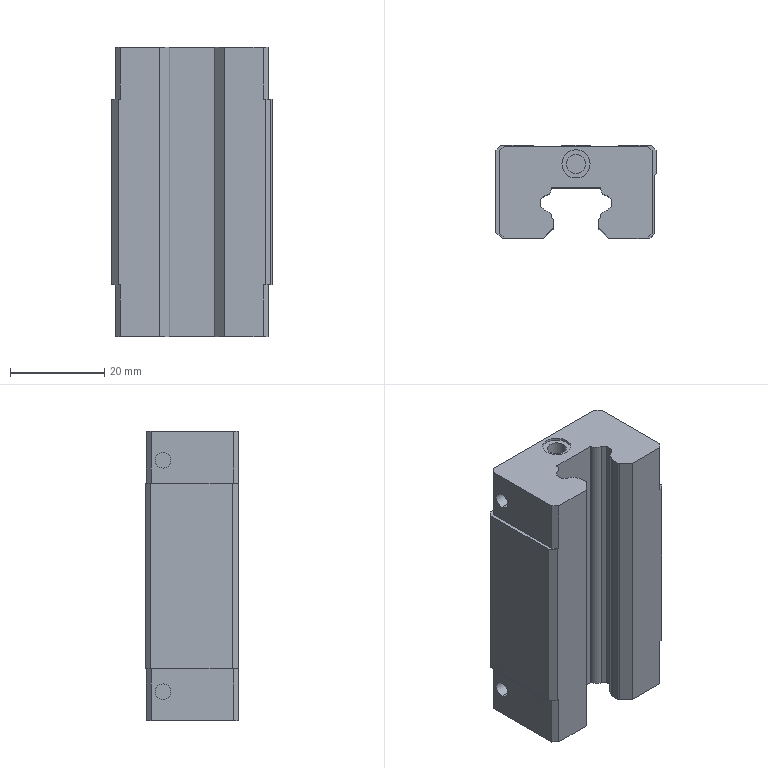Part | STEP file | HGH15_2 | 1 solid | 124 faces | box 34 x 19.7 x 61.4 mm | volume 31145 mm3 | plane 72 | cylinder 44 | cone 8 | commonest cylinder face diameters 3.3 x16 0.8 x8 1 x4 3.24 x4 4 x4 5.3 x4